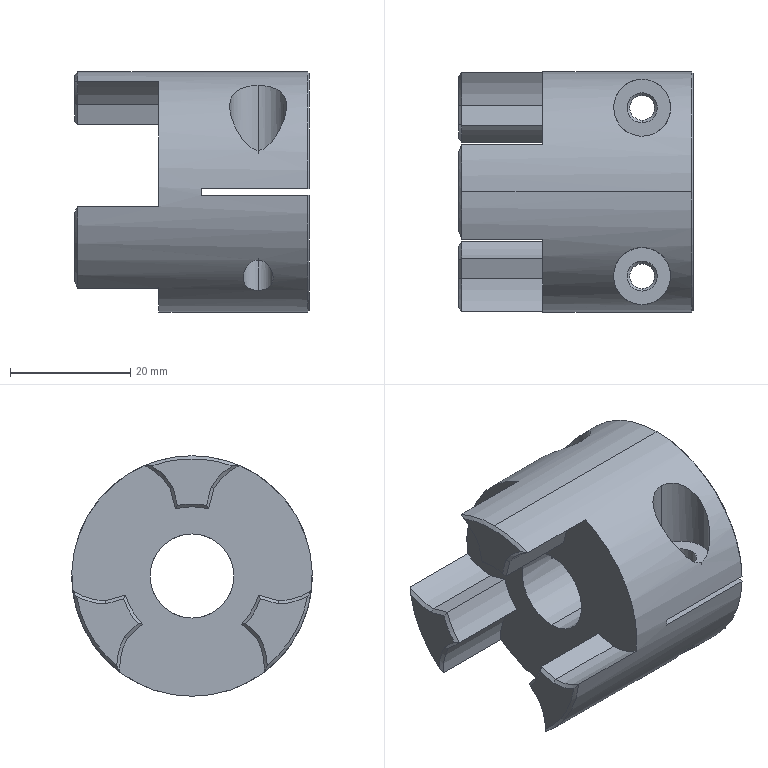Part | STEP file | R_CPJC40_14 | 1 solid | 79 faces | box 39 x 40 x 40 mm | volume 28571 mm3 | cylinder 30 | plane 26 | cone 23 | commonest cylinder face diameters 5 x8 19.758 x6 4.134 x4 9.5 x4 23 x4 14 x2